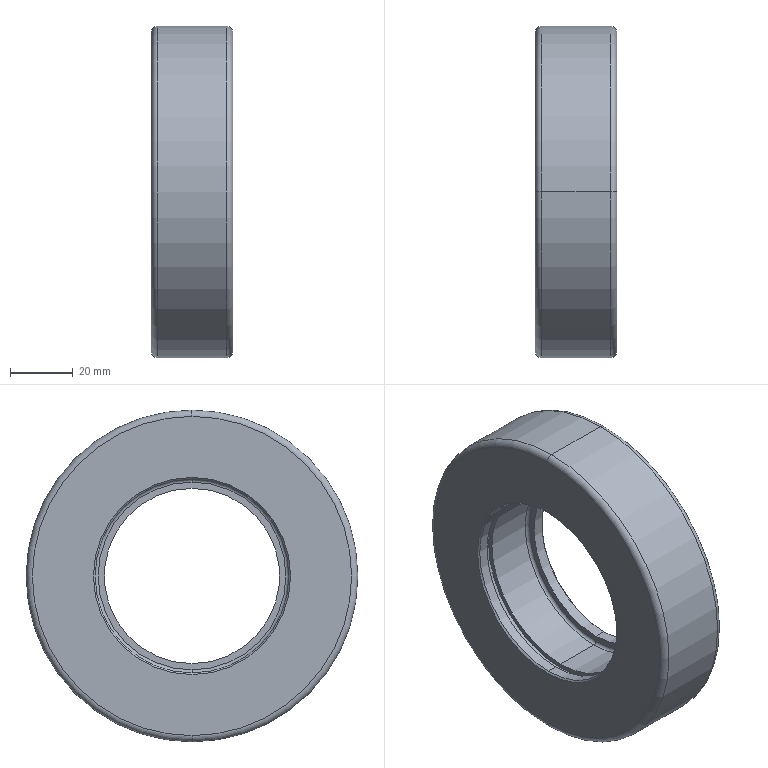Part | STEP file | BT2022003-01-10 Guide wheel A | 1 solid | 25 faces | box 26 x 106 x 106 mm | volume 151941 mm3 | cylinder 10 | torus 6 | plane 5 | cone 4 | commonest cylinder face diameters 62 x4 56 x2 65 x2 106 x2
STEP:
#1=CARTESIAN_POINT('',(0.5,0.,-31.));
#2=VERTEX_POINT('',#1);
#3=CARTESIAN_POINT('',(0.5,0.,31.));
#4=VERTEX_POINT('',#3);
#5=CARTESIAN_POINT('',(0.5,0.,0.));
#6=DIRECTION('',(-1.,0.,0.));
#7=DIRECTION('',(0.,0.,-1.));
#8=AXIS2_PLACEMENT_3D('',#5,#6,#7);
#9=CIRCLE('',#8,31.);
#10=EDGE_CURVE('',#2,#4,#9,.T.);
#11=ORIENTED_EDGE('',*,*,#10,.F.);
#12=CARTESIAN_POINT('',(0.,0.,-31.5));
#13=VERTEX_POINT('',#12);
#14=CARTESIAN_POINT('',(0.5,0.,-31.));
#15=DIRECTION('',(-0.7071,0.,-0.7071));
#16=VECTOR('',#15,1000.);
#17=LINE('',#14,#16);
#18=EDGE_CURVE('',#2,#13,#17,.T.);
#19=ORIENTED_EDGE('',*,*,#18,.T.);
#20=CARTESIAN_POINT('',(0.,0.,31.5));
#21=VERTEX_POINT('',#20);
#22=CARTESIAN_POINT('',(0.,0.,0.));
#23=DIRECTION('',(1.,0.,0.));
#24=DIRECTION('',(0.,0.,-1.));
#25=AXIS2_PLACEMENT_3D('',#22,#23,#24);
#26=CIRCLE('',#25,31.5);
#27=EDGE_CURVE('',#21,#13,#26,.T.);
#28=ORIENTED_EDGE('',*,*,#27,.F.);
#29=CARTESIAN_POINT('',(0.5,0.,31.));
#30=DIRECTION('',(-0.7071,0.,0.7071));
#31=VECTOR('',#30,1000.);
#32=LINE('',#29,#31);
#33=EDGE_CURVE('',#4,#21,#32,.T.);
#34=ORIENTED_EDGE('',*,*,#33,.F.);
#35=EDGE_LOOP('',(#11,#19,#28,#34));
#36=FACE_OUTER_BOUND('',#35,.T.);
#37=CARTESIAN_POINT('',(0.5,0.,0.));
#38=DIRECTION('',(-1.,0.,0.));
#39=DIRECTION('',(0.,0.,1.));
#40=AXIS2_PLACEMENT_3D('',#37,#38,#39);
#41=CONICAL_SURFACE('',#40,31.,0.7854);
#42=ADVANCED_FACE('',(#36),#41,.F.);
#43=CARTESIAN_POINT('',(25.5,0.,28.));
#44=VERTEX_POINT('',#43);
#45=CARTESIAN_POINT('',(25.5,0.,-28.));
#46=VERTEX_POINT('',#45);
#47=CARTESIAN_POINT('',(25.5,0.,0.));
#48=DIRECTION('',(1.,0.,0.));
#49=DIRECTION('',(0.,0.,1.));
#50=AXIS2_PLACEMENT_3D('',#47,#48,#49);
#51=CIRCLE('',#50,28.);
#52=EDGE_CURVE('',#44,#46,#51,.T.);
#53=ORIENTED_EDGE('',*,*,#52,.F.);
#54=CARTESIAN_POINT('',(26.,0.,28.5));
#55=VERTEX_POINT('',#54);
#56=CARTESIAN_POINT('',(26.,0.,28.5));
#57=DIRECTION('',(0.7071,0.,0.7071));
#58=VECTOR('',#57,1000.);
#59=LINE('',#56,#58);
#60=EDGE_CURVE('',#44,#55,#59,.T.);
#61=ORIENTED_EDGE('',*,*,#60,.T.);
#62=CARTESIAN_POINT('',(26.,0.,-28.5));
#63=VERTEX_POINT('',#62);
#64=CARTESIAN_POINT('',(26.,0.,0.));
#65=DIRECTION('',(-1.,0.,0.));
#66=DIRECTION('',(0.,0.,1.));
#67=AXIS2_PLACEMENT_3D('',#64,#65,#66);
#68=CIRCLE('',#67,28.5);
#69=EDGE_CURVE('',#63,#55,#68,.T.);
#70=ORIENTED_EDGE('',*,*,#69,.F.);
#71=CARTESIAN_POINT('',(26.,0.,-28.5));
#72=DIRECTION('',(0.7071,0.,-0.7071));
#73=VECTOR('',#72,1000.);
#74=LINE('',#71,#73);
#75=EDGE_CURVE('',#46,#63,#74,.T.);
#76=ORIENTED_EDGE('',*,*,#75,.F.);
#77=EDGE_LOOP('',(#53,#61,#70,#76));
#78=FACE_OUTER_BOUND('',#77,.T.);
#79=CARTESIAN_POINT('',(26.,0.,0.));
#80=DIRECTION('',(1.,0.,0.));
#81=DIRECTION('',(0.,0.,-1.));
#82=AXIS2_PLACEMENT_3D('',#79,#80,#81);
#83=CONICAL_SURFACE('',#82,28.5,0.7854);
#84=ADVANCED_FACE('',(#78),#83,.F.);
#85=CARTESIAN_POINT('',(26.,0.,-51.));
#86=VERTEX_POINT('',#85);
#87=CARTESIAN_POINT('',(26.,0.,51.));
#88=VERTEX_POINT('',#87);
#89=CARTESIAN_POINT('',(26.,0.,0.));
#90=DIRECTION('',(1.,0.,0.));
#91=DIRECTION('',(0.,0.,1.));
#92=AXIS2_PLACEMENT_3D('',#89,#90,#91);
#93=CIRCLE('',#92,51.);
#94=EDGE_CURVE('',#86,#88,#93,.T.);
#95=ORIENTED_EDGE('',*,*,#94,.F.);
#96=CARTESIAN_POINT('',(24.,0.,-53.));
#97=VERTEX_POINT('',#96);
#98=CARTESIAN_POINT('',(24.,0.,-51.));
#99=DIRECTION('',(0.,1.,0.));
#100=DIRECTION('',(0.,0.,1.));
#101=AXIS2_PLACEMENT_3D('',#98,#99,#100);
#102=CIRCLE('',#101,2.);
#103=EDGE_CURVE('',#86,#97,#102,.T.);
#104=ORIENTED_EDGE('',*,*,#103,.T.);
#105=CARTESIAN_POINT('',(24.,0.,53.));
#106=VERTEX_POINT('',#105);
#107=CARTESIAN_POINT('',(24.,0.,0.));
#108=DIRECTION('',(-1.,0.,0.));
#109=DIRECTION('',(0.,0.,1.));
#110=AXIS2_PLACEMENT_3D('',#107,#108,#109);
#111=CIRCLE('',#110,53.);
#112=EDGE_CURVE('',#106,#97,#111,.T.);
#113=ORIENTED_EDGE('',*,*,#112,.F.);
#114=CARTESIAN_POINT('',(24.,0.,51.));
#115=DIRECTION('',(0.,-1.,0.));
#116=DIRECTION('',(0.,0.,-1.));
#117=AXIS2_PLACEMENT_3D('',#114,#115,#116);
#118=CIRCLE('',#117,2.);
#119=EDGE_CURVE('',#88,#106,#118,.T.);
#120=ORIENTED_EDGE('',*,*,#119,.F.);
#121=EDGE_LOOP('',(#95,#104,#113,#120));
#122=FACE_OUTER_BOUND('',#121,.T.);
#123=CARTESIAN_POINT('',(24.,0.,0.));
#124=DIRECTION('',(-1.,0.,0.));
#125=DIRECTION('',(0.,0.,1.));
#126=AXIS2_PLACEMENT_3D('',#123,#124,#125);
#127=TOROIDAL_SURFACE('',#126,51.,2.);
#128=ADVANCED_FACE('',(#122),#127,.T.);
#129=CARTESIAN_POINT('',(0.,0.,51.));
#130=VERTEX_POINT('',#129);
#131=CARTESIAN_POINT('',(0.,0.,-51.));
#132=VERTEX_POINT('',#131);
#133=CARTESIAN_POINT('',(0.,0.,0.));
#134=DIRECTION('',(-1.,0.,0.));
#135=DIRECTION('',(0.,0.,-1.));
#136=AXIS2_PLACEMENT_3D('',#133,#134,#135);
#137=CIRCLE('',#136,51.);
#138=EDGE_CURVE('',#130,#132,#137,.T.);
#139=ORIENTED_EDGE('',*,*,#138,.F.);
#140=CARTESIAN_POINT('',(2.,0.,53.));
#141=VERTEX_POINT('',#140);
#142=CARTESIAN_POINT('',(2.,0.,51.));
#143=DIRECTION('',(0.,1.,0.));
#144=DIRECTION('',(0.,0.,1.));
#145=AXIS2_PLACEMENT_3D('',#142,#143,#144);
#146=CIRCLE('',#145,2.);
#147=EDGE_CURVE('',#130,#141,#146,.T.);
#148=ORIENTED_EDGE('',*,*,#147,.T.);
#149=CARTESIAN_POINT('',(2.,0.,-53.));
#150=VERTEX_POINT('',#149);
#151=CARTESIAN_POINT('',(2.,0.,0.));
#152=DIRECTION('',(1.,0.,0.));
#153=DIRECTION('',(0.,0.,-1.));
#154=AXIS2_PLACEMENT_3D('',#151,#152,#153);
#155=CIRCLE('',#154,53.);
#156=EDGE_CURVE('',#150,#141,#155,.T.);
#157=ORIENTED_EDGE('',*,*,#156,.F.);
#158=CARTESIAN_POINT('',(2.,0.,-51.));
#159=DIRECTION('',(0.,-1.,0.));
#160=DIRECTION('',(0.,0.,-1.));
#161=AXIS2_PLACEMENT_3D('',#158,#159,#160);
#162=CIRCLE('',#161,2.);
#163=EDGE_CURVE('',#132,#150,#162,.T.);
#164=ORIENTED_EDGE('',*,*,#163,.F.);
#165=EDGE_LOOP('',(#139,#148,#157,#164));
#166=FACE_OUTER_BOUND('',#165,.T.);
#167=CARTESIAN_POINT('',(2.,0.,0.));
#168=DIRECTION('',(1.,0.,0.));
#169=DIRECTION('',(0.,0.,-1.));
#170=AXIS2_PLACEMENT_3D('',#167,#168,#169);
#171=TOROIDAL_SURFACE('',#170,51.,2.);
#172=ADVANCED_FACE('',(#166),#171,.T.);
#173=ORIENTED_EDGE('',*,*,#52,.T.);
#174=CARTESIAN_POINT('',(22.,0.,-28.));
#175=VERTEX_POINT('',#174);
#176=CARTESIAN_POINT('',(0.,0.,-28.));
#177=DIRECTION('',(-1.,0.,0.));
#178=VECTOR('',#177,1000.);
#179=LINE('',#176,#178);
#180=EDGE_CURVE('',#46,#175,#179,.T.);
#181=ORIENTED_EDGE('',*,*,#180,.T.);
#182=CARTESIAN_POINT('',(22.,0.,28.));
#183=VERTEX_POINT('',#182);
#184=CARTESIAN_POINT('',(22.,0.,0.));
#185=DIRECTION('',(-1.,0.,0.));
#186=DIRECTION('',(0.,0.,1.));
#187=AXIS2_PLACEMENT_3D('',#184,#185,#186);
#188=CIRCLE('',#187,28.);
#189=EDGE_CURVE('',#175,#183,#188,.T.);
#190=ORIENTED_EDGE('',*,*,#189,.T.);
#191=CARTESIAN_POINT('',(0.,0.,28.));
#192=DIRECTION('',(-1.,0.,0.));
#193=VECTOR('',#192,1000.);
#194=LINE('',#191,#193);
#195=EDGE_CURVE('',#44,#183,#194,.T.);
#196=ORIENTED_EDGE('',*,*,#195,.F.);
#197=EDGE_LOOP('',(#173,#181,#190,#196));
#198=FACE_OUTER_BOUND('',#197,.T.);
#199=CARTESIAN_POINT('',(0.,0.,0.));
#200=DIRECTION('',(-1.,0.,0.));
#201=DIRECTION('',(0.,0.,1.));
#202=AXIS2_PLACEMENT_3D('',#199,#200,#201);
#203=CYLINDRICAL_SURFACE('',#202,28.);
#204=ADVANCED_FACE('',(#198),#203,.F.);
#205=ORIENTED_EDGE('',*,*,#112,.T.);
#206=CARTESIAN_POINT('',(0.,0.,-53.));
#207=DIRECTION('',(-1.,0.,0.));
#208=VECTOR('',#207,1000.);
#209=LINE('',#206,#208);
#210=EDGE_CURVE('',#97,#150,#209,.T.);
#211=ORIENTED_EDGE('',*,*,#210,.T.);
#212=ORIENTED_EDGE('',*,*,#156,.T.);
#213=CARTESIAN_POINT('',(0.,0.,53.));
#214=DIRECTION('',(-1.,0.,0.));
#215=VECTOR('',#214,1000.);
#216=LINE('',#213,#215);
#217=EDGE_CURVE('',#106,#141,#216,.T.);
#218=ORIENTED_EDGE('',*,*,#217,.F.);
#219=EDGE_LOOP('',(#205,#211,#212,#218));
#220=FACE_OUTER_BOUND('',#219,.T.);
#221=CARTESIAN_POINT('',(0.,0.,0.));
#222=DIRECTION('',(-1.,0.,0.));
#223=DIRECTION('',(0.,0.,1.));
#224=AXIS2_PLACEMENT_3D('',#221,#222,#223);
#225=CYLINDRICAL_SURFACE('',#224,53.);
#226=ADVANCED_FACE('',(#220),#225,.T.);
#227=CARTESIAN_POINT('',(3.8,0.,-31.));
#228=VERTEX_POINT('',#227);
#229=CARTESIAN_POINT('',(3.8,0.,31.));
#230=VERTEX_POINT('',#229);
#231=CARTESIAN_POINT('',(3.8,0.,0.));
#232=DIRECTION('',(-1.,0.,0.));
#233=DIRECTION('',(0.,0.,1.));
#234=AXIS2_PLACEMENT_3D('',#231,#232,#233);
#235=CIRCLE('',#234,31.);
#236=EDGE_CURVE('',#228,#230,#235,.T.);
#237=ORIENTED_EDGE('',*,*,#236,.F.);
#238=CARTESIAN_POINT('',(0.,0.,-31.));
#239=DIRECTION('',(-1.,0.,0.));
#240=VECTOR('',#239,1000.);
#241=LINE('',#238,#240);
#242=EDGE_CURVE('',#228,#2,#241,.T.);
#243=ORIENTED_EDGE('',*,*,#242,.T.);
#244=ORIENTED_EDGE('',*,*,#10,.T.);
#245=CARTESIAN_POINT('',(0.,0.,31.));
#246=DIRECTION('',(-1.,0.,0.));
#247=VECTOR('',#246,1000.);
#248=LINE('',#245,#247);
#249=EDGE_CURVE('',#230,#4,#248,.T.);
#250=ORIENTED_EDGE('',*,*,#249,.F.);
#251=EDGE_LOOP('',(#237,#243,#244,#250));
#252=FACE_OUTER_BOUND('',#251,.T.);
#253=CARTESIAN_POINT('',(0.,0.,0.));
#254=DIRECTION('',(-1.,0.,0.));
#255=DIRECTION('',(0.,0.,1.));
#256=AXIS2_PLACEMENT_3D('',#253,#254,#255);
#257=CYLINDRICAL_SURFACE('',#256,31.);
#258=ADVANCED_FACE('',(#252),#257,.F.);
#259=CARTESIAN_POINT('',(6.,0.,-32.5));
#260=VERTEX_POINT('',#259);
#261=CARTESIAN_POINT('',(6.,0.,32.5));
#262=VERTEX_POINT('',#261);
#263=CARTESIAN_POINT('',(6.,0.,0.));
#264=DIRECTION('',(-1.,0.,0.));
#265=DIRECTION('',(0.,0.,1.));
#266=AXIS2_PLACEMENT_3D('',#263,#264,#265);
#267=CIRCLE('',#266,32.5);
#268=EDGE_CURVE('',#260,#262,#267,.T.);
#269=ORIENTED_EDGE('',*,*,#268,.F.);
#270=CARTESIAN_POINT('',(3.8,0.,-32.5));
#271=VERTEX_POINT('',#270);
#272=CARTESIAN_POINT('',(0.,0.,-32.5));
#273=DIRECTION('',(-1.,0.,0.));
#274=VECTOR('',#273,1000.);
#275=LINE('',#272,#274);
#276=EDGE_CURVE('',#260,#271,#275,.T.);
#277=ORIENTED_EDGE('',*,*,#276,.T.);
#278=CARTESIAN_POINT('',(3.8,0.,32.5));
#279=VERTEX_POINT('',#278);
#280=CARTESIAN_POINT('',(3.8,0.,0.));
#281=DIRECTION('',(-1.,0.,0.));
#282=DIRECTION('',(0.,0.,1.));
#283=AXIS2_PLACEMENT_3D('',#280,#281,#282);
#284=CIRCLE('',#283,32.5);
#285=EDGE_CURVE('',#271,#279,#284,.T.);
#286=ORIENTED_EDGE('',*,*,#285,.T.);
#287=CARTESIAN_POINT('',(0.,0.,32.5));
#288=DIRECTION('',(-1.,0.,0.));
#289=VECTOR('',#288,1000.);
#290=LINE('',#287,#289);
#291=EDGE_CURVE('',#262,#279,#290,.T.);
#292=ORIENTED_EDGE('',*,*,#291,.F.);
#293=EDGE_LOOP('',(#269,#277,#286,#292));
#294=FACE_OUTER_BOUND('',#293,.T.);
#295=CARTESIAN_POINT('',(0.,0.,0.));
#296=DIRECTION('',(-1.,0.,0.));
#297=DIRECTION('',(0.,0.,1.));
#298=AXIS2_PLACEMENT_3D('',#295,#296,#297);
#299=CYLINDRICAL_SURFACE('',#298,32.5);
#300=ADVANCED_FACE('',(#294),#299,.F.);
#301=CARTESIAN_POINT('',(21.,0.,-31.));
#302=VERTEX_POINT('',#301);
#303=CARTESIAN_POINT('',(21.,0.,31.));
#304=VERTEX_POINT('',#303);
#305=CARTESIAN_POINT('',(21.,0.,0.));
#306=DIRECTION('',(-1.,0.,0.));
#307=DIRECTION('',(0.,0.,1.));
#308=AXIS2_PLACEMENT_3D('',#305,#306,#307);
#309=CIRCLE('',#308,31.);
#310=EDGE_CURVE('',#302,#304,#309,.T.);
#311=ORIENTED_EDGE('',*,*,#310,.F.);
#312=CARTESIAN_POINT('',(6.,0.,-31.));
#313=VERTEX_POINT('',#312);
#314=CARTESIAN_POINT('',(0.,0.,-31.));
#315=DIRECTION('',(-1.,0.,0.));
#316=VECTOR('',#315,1000.);
#317=LINE('',#314,#316);
#318=EDGE_CURVE('',#302,#313,#317,.T.);
#319=ORIENTED_EDGE('',*,*,#318,.T.);
#320=CARTESIAN_POINT('',(6.,0.,31.));
#321=VERTEX_POINT('',#320);
#322=CARTESIAN_POINT('',(6.,0.,0.));
#323=DIRECTION('',(-1.,0.,0.));
#324=DIRECTION('',(0.,0.,1.));
#325=AXIS2_PLACEMENT_3D('',#322,#323,#324);
#326=CIRCLE('',#325,31.);
#327=EDGE_CURVE('',#313,#321,#326,.T.);
#328=ORIENTED_EDGE('',*,*,#327,.T.);
#329=CARTESIAN_POINT('',(0.,0.,31.));
#330=DIRECTION('',(-1.,0.,0.));
#331=VECTOR('',#330,1000.);
#332=LINE('',#329,#331);
#333=EDGE_CURVE('',#304,#321,#332,.T.);
#334=ORIENTED_EDGE('',*,*,#333,.F.);
#335=EDGE_LOOP('',(#311,#319,#328,#334));
#336=FACE_OUTER_BOUND('',#335,.T.);
#337=CARTESIAN_POINT('',(0.,0.,0.));
#338=DIRECTION('',(-1.,0.,0.));
#339=DIRECTION('',(0.,0.,1.));
#340=AXIS2_PLACEMENT_3D('',#337,#338,#339);
#341=CYLINDRICAL_SURFACE('',#340,31.);
#342=ADVANCED_FACE('',(#336),#341,.F.);
#343=CARTESIAN_POINT('',(22.,0.,-30.));
#344=VERTEX_POINT('',#343);
#345=CARTESIAN_POINT('',(22.,0.,30.));
#346=VERTEX_POINT('',#345);
#347=CARTESIAN_POINT('',(22.,0.,0.));
#348=DIRECTION('',(-1.,0.,0.));
#349=DIRECTION('',(0.,0.,1.));
#350=AXIS2_PLACEMENT_3D('',#347,#348,#349);
#351=CIRCLE('',#350,30.);
#352=EDGE_CURVE('',#344,#346,#351,.T.);
#353=ORIENTED_EDGE('',*,*,#352,.F.);
#354=CARTESIAN_POINT('',(21.,0.,-30.));
#355=DIRECTION('',(0.,1.,0.));
#356=DIRECTION('',(0.,0.,1.));
#357=AXIS2_PLACEMENT_3D('',#354,#355,#356);
#358=CIRCLE('',#357,1.);
#359=EDGE_CURVE('',#344,#302,#358,.T.);
#360=ORIENTED_EDGE('',*,*,#359,.T.);
#361=ORIENTED_EDGE('',*,*,#310,.T.);
#362=CARTESIAN_POINT('',(21.,0.,30.));
#363=DIRECTION('',(0.,-1.,0.));
#364=DIRECTION('',(0.,0.,-1.));
#365=AXIS2_PLACEMENT_3D('',#362,#363,#364);
#366=CIRCLE('',#365,1.);
#367=EDGE_CURVE('',#346,#304,#366,.T.);
#368=ORIENTED_EDGE('',*,*,#367,.F.);
#369=EDGE_LOOP('',(#353,#360,#361,#368));
#370=FACE_OUTER_BOUND('',#369,.T.);
#371=CARTESIAN_POINT('',(21.,0.,0.));
#372=DIRECTION('',(-1.,0.,0.));
#373=DIRECTION('',(0.,0.,1.));
#374=AXIS2_PLACEMENT_3D('',#371,#372,#373);
#375=TOROIDAL_SURFACE('',#374,30.,1.);
#376=ADVANCED_FACE('',(#370),#375,.F.);
#377=ORIENTED_EDGE('',*,*,#359,.F.);
#378=CARTESIAN_POINT('',(22.,0.,0.));
#379=DIRECTION('',(-1.,0.,0.));
#380=DIRECTION('',(0.,0.,1.));
#381=AXIS2_PLACEMENT_3D('',#378,#379,#380);
#382=CIRCLE('',#381,30.);
#383=EDGE_CURVE('',#346,#344,#382,.T.);
#384=ORIENTED_EDGE('',*,*,#383,.F.);
#385=ORIENTED_EDGE('',*,*,#367,.T.);
#386=CARTESIAN_POINT('',(21.,0.,0.));
#387=DIRECTION('',(-1.,0.,0.));
#388=DIRECTION('',(0.,0.,1.));
#389=AXIS2_PLACEMENT_3D('',#386,#387,#388);
#390=CIRCLE('',#389,31.);
#391=EDGE_CURVE('',#304,#302,#390,.T.);
#392=ORIENTED_EDGE('',*,*,#391,.T.);
#393=EDGE_LOOP('',(#377,#384,#385,#392));
#394=FACE_OUTER_BOUND('',#393,.T.);
#395=CARTESIAN_POINT('',(21.,0.,0.));
#396=DIRECTION('',(-1.,0.,0.));
#397=DIRECTION('',(0.,0.,1.));
#398=AXIS2_PLACEMENT_3D('',#395,#396,#397);
#399=TOROIDAL_SURFACE('',#398,30.,1.);
#400=ADVANCED_FACE('',(#394),#399,.F.);
#401=ORIENTED_EDGE('',*,*,#318,.F.);
#402=ORIENTED_EDGE('',*,*,#391,.F.);
#403=ORIENTED_EDGE('',*,*,#333,.T.);
#404=CARTESIAN_POINT('',(6.,0.,0.));
#405=DIRECTION('',(-1.,0.,0.));
#406=DIRECTION('',(0.,0.,1.));
#407=AXIS2_PLACEMENT_3D('',#404,#405,#406);
#408=CIRCLE('',#407,31.);
#409=EDGE_CURVE('',#321,#313,#408,.T.);
#410=ORIENTED_EDGE('',*,*,#409,.T.);
#411=EDGE_LOOP('',(#401,#402,#403,#410));
#412=FACE_OUTER_BOUND('',#411,.T.);
#413=CARTESIAN_POINT('',(0.,0.,0.));
#414=DIRECTION('',(-1.,0.,0.));
#415=DIRECTION('',(0.,0.,1.));
#416=AXIS2_PLACEMENT_3D('',#413,#414,#415);
#417=CYLINDRICAL_SURFACE('',#416,31.);
#418=ADVANCED_FACE('',(#412),#417,.F.);
#419=ORIENTED_EDGE('',*,*,#409,.F.);
#420=ORIENTED_EDGE('',*,*,#327,.F.);
#421=EDGE_LOOP('',(#419,#420));
#422=FACE_BOUND('',#421,.T.);
#423=CARTESIAN_POINT('',(6.,0.,0.));
#424=DIRECTION('',(-1.,0.,0.));
#425=DIRECTION('',(0.,0.,1.));
#426=AXIS2_PLACEMENT_3D('',#423,#424,#425);
#427=CIRCLE('',#426,32.5);
#428=EDGE_CURVE('',#262,#260,#427,.T.);
#429=ORIENTED_EDGE('',*,*,#428,.T.);
#430=ORIENTED_EDGE('',*,*,#268,.T.);
#431=EDGE_LOOP('',(#429,#430));
#432=FACE_OUTER_BOUND('',#431,.T.);
#433=CARTESIAN_POINT('',(6.,32.5,0.));
#434=DIRECTION('',(1.,0.,0.));
#435=DIRECTION('',(0.,0.,-1.));
#436=AXIS2_PLACEMENT_3D('',#433,#434,#435);
#437=PLANE('',#436);
#438=ADVANCED_FACE('',(#422,#432),#437,.F.);
#439=ORIENTED_EDGE('',*,*,#276,.F.);
#440=ORIENTED_EDGE('',*,*,#428,.F.);
#441=ORIENTED_EDGE('',*,*,#291,.T.);
#442=CARTESIAN_POINT('',(3.8,0.,0.));
#443=DIRECTION('',(-1.,0.,0.));
#444=DIRECTION('',(0.,0.,1.));
#445=AXIS2_PLACEMENT_3D('',#442,#443,#444);
#446=CIRCLE('',#445,32.5);
#447=EDGE_CURVE('',#279,#271,#446,.T.);
#448=ORIENTED_EDGE('',*,*,#447,.T.);
#449=EDGE_LOOP('',(#439,#440,#441,#448));
#450=FACE_OUTER_BOUND('',#449,.T.);
#451=CARTESIAN_POINT('',(0.,0.,0.));
#452=DIRECTION('',(-1.,0.,0.));
#453=DIRECTION('',(0.,0.,1.));
#454=AXIS2_PLACEMENT_3D('',#451,#452,#453);
#455=CYLINDRICAL_SURFACE('',#454,32.5);
#456=ADVANCED_FACE('',(#450),#455,.F.);
#457=ORIENTED_EDGE('',*,*,#447,.F.);
#458=ORIENTED_EDGE('',*,*,#285,.F.);
#459=EDGE_LOOP('',(#457,#458));
#460=FACE_OUTER_BOUND('',#459,.T.);
#461=CARTESIAN_POINT('',(3.8,0.,0.));
#462=DIRECTION('',(-1.,0.,0.));
#463=DIRECTION('',(0.,0.,1.));
#464=AXIS2_PLACEMENT_3D('',#461,#462,#463);
#465=CIRCLE('',#464,31.);
#466=EDGE_CURVE('',#230,#228,#465,.T.);
#467=ORIENTED_EDGE('',*,*,#466,.T.);
#468=ORIENTED_EDGE('',*,*,#236,.T.);
#469=EDGE_LOOP('',(#467,#468));
#470=FACE_BOUND('',#469,.T.);
#471=CARTESIAN_POINT('',(3.8,31.,0.));
#472=DIRECTION('',(-1.,0.,0.));
#473=DIRECTION('',(0.,0.,1.));
#474=AXIS2_PLACEMENT_3D('',#471,#472,#473);
#475=PLANE('',#474);
#476=ADVANCED_FACE('',(#460,#470),#475,.F.);
#477=ORIENTED_EDGE('',*,*,#242,.F.);
#478=ORIENTED_EDGE('',*,*,#466,.F.);
#479=ORIENTED_EDGE('',*,*,#249,.T.);
#480=CARTESIAN_POINT('',(0.5,0.,0.));
#481=DIRECTION('',(-1.,0.,0.));
#482=DIRECTION('',(0.,0.,-1.));
#483=AXIS2_PLACEMENT_3D('',#480,#481,#482);
#484=CIRCLE('',#483,31.);
#485=EDGE_CURVE('',#4,#2,#484,.T.);
#486=ORIENTED_EDGE('',*,*,#485,.T.);
#487=EDGE_LOOP('',(#477,#478,#479,#486));
#488=FACE_OUTER_BOUND('',#487,.T.);
#489=CARTESIAN_POINT('',(0.,0.,0.));
#490=DIRECTION('',(-1.,0.,0.));
#491=DIRECTION('',(0.,0.,1.));
#492=AXIS2_PLACEMENT_3D('',#489,#490,#491);
#493=CYLINDRICAL_SURFACE('',#492,31.);
#494=ADVANCED_FACE('',(#488),#493,.F.);
#495=ORIENTED_EDGE('',*,*,#27,.T.);
#496=CARTESIAN_POINT('',(0.,0.,0.));
#497=DIRECTION('',(1.,0.,0.));
#498=DIRECTION('',(0.,0.,-1.));
#499=AXIS2_PLACEMENT_3D('',#496,#497,#498);
#500=CIRCLE('',#499,31.5);
#501=EDGE_CURVE('',#13,#21,#500,.T.);
#502=ORIENTED_EDGE('',*,*,#501,.T.);
#503=EDGE_LOOP('',(#495,#502));
#504=FACE_BOUND('',#503,.T.);
#505=CARTESIAN_POINT('',(0.,0.,0.));
#506=DIRECTION('',(-1.,0.,0.));
#507=DIRECTION('',(0.,0.,-1.));
#508=AXIS2_PLACEMENT_3D('',#505,#506,#507);
#509=CIRCLE('',#508,51.);
#510=EDGE_CURVE('',#132,#130,#509,.T.);
#511=ORIENTED_EDGE('',*,*,#510,.T.);
#512=ORIENTED_EDGE('',*,*,#138,.T.);
#513=EDGE_LOOP('',(#511,#512));
#514=FACE_OUTER_BOUND('',#513,.T.);
#515=CARTESIAN_POINT('',(0.,53.,0.));
#516=DIRECTION('',(1.,0.,0.));
#517=DIRECTION('',(0.,0.,-1.));
#518=AXIS2_PLACEMENT_3D('',#515,#516,#517);
#519=PLANE('',#518);
#520=ADVANCED_FACE('',(#504,#514),#519,.F.);
#521=ORIENTED_EDGE('',*,*,#210,.F.);
#522=CARTESIAN_POINT('',(24.,0.,0.));
#523=DIRECTION('',(-1.,0.,0.));
#524=DIRECTION('',(0.,0.,1.));
#525=AXIS2_PLACEMENT_3D('',#522,#523,#524);
#526=CIRCLE('',#525,53.);
#527=EDGE_CURVE('',#97,#106,#526,.T.);
#528=ORIENTED_EDGE('',*,*,#527,.T.);
#529=ORIENTED_EDGE('',*,*,#217,.T.);
#530=CARTESIAN_POINT('',(2.,0.,0.));
#531=DIRECTION('',(1.,0.,0.));
#532=DIRECTION('',(0.,0.,-1.));
#533=AXIS2_PLACEMENT_3D('',#530,#531,#532);
#534=CIRCLE('',#533,53.);
#535=EDGE_CURVE('',#141,#150,#534,.T.);
#536=ORIENTED_EDGE('',*,*,#535,.T.);
#537=EDGE_LOOP('',(#521,#528,#529,#536));
#538=FACE_OUTER_BOUND('',#537,.T.);
#539=CARTESIAN_POINT('',(0.,0.,0.));
#540=DIRECTION('',(-1.,0.,0.));
#541=DIRECTION('',(0.,0.,1.));
#542=AXIS2_PLACEMENT_3D('',#539,#540,#541);
#543=CYLINDRICAL_SURFACE('',#542,53.);
#544=ADVANCED_FACE('',(#538),#543,.T.);
#545=ORIENTED_EDGE('',*,*,#69,.T.);
#546=CARTESIAN_POINT('',(26.,0.,0.));
#547=DIRECTION('',(-1.,0.,0.));
#548=DIRECTION('',(0.,0.,1.));
#549=AXIS2_PLACEMENT_3D('',#546,#547,#548);
#550=CIRCLE('',#549,28.5);
#551=EDGE_CURVE('',#55,#63,#550,.T.);
#552=ORIENTED_EDGE('',*,*,#551,.T.);
#553=EDGE_LOOP('',(#545,#552));
#554=FACE_BOUND('',#553,.T.);
#555=CARTESIAN_POINT('',(26.,0.,0.));
#556=DIRECTION('',(1.,0.,0.));
#557=DIRECTION('',(0.,0.,1.));
#558=AXIS2_PLACEMENT_3D('',#555,#556,#557);
#559=CIRCLE('',#558,51.);
#560=EDGE_CURVE('',#88,#86,#559,.T.);
#561=ORIENTED_EDGE('',*,*,#560,.T.);
#562=ORIENTED_EDGE('',*,*,#94,.T.);
#563=EDGE_LOOP('',(#561,#562));
#564=FACE_OUTER_BOUND('',#563,.T.);
#565=CARTESIAN_POINT('',(26.,28.,0.));
#566=DIRECTION('',(-1.,0.,0.));
#567=DIRECTION('',(0.,0.,1.));
#568=AXIS2_PLACEMENT_3D('',#565,#566,#567);
#569=PLANE('',#568);
#570=ADVANCED_FACE('',(#554,#564),#569,.F.);
#571=ORIENTED_EDGE('',*,*,#180,.F.);
#572=CARTESIAN_POINT('',(25.5,0.,0.));
#573=DIRECTION('',(1.,0.,0.));
#574=DIRECTION('',(0.,0.,1.));
#575=AXIS2_PLACEMENT_3D('',#572,#573,#574);
#576=CIRCLE('',#575,28.);
#577=EDGE_CURVE('',#46,#44,#576,.T.);
#578=ORIENTED_EDGE('',*,*,#577,.T.);
#579=ORIENTED_EDGE('',*,*,#195,.T.);
#580=CARTESIAN_POINT('',(22.,0.,0.));
#581=DIRECTION('',(-1.,0.,0.));
#582=DIRECTION('',(0.,0.,1.));
#583=AXIS2_PLACEMENT_3D('',#580,#581,#582);
#584=CIRCLE('',#583,28.);
#585=EDGE_CURVE('',#183,#175,#584,.T.);
#586=ORIENTED_EDGE('',*,*,#585,.T.);
#587=EDGE_LOOP('',(#571,#578,#579,#586));
#588=FACE_OUTER_BOUND('',#587,.T.);
#589=CARTESIAN_POINT('',(0.,0.,0.));
#590=DIRECTION('',(-1.,0.,0.));
#591=DIRECTION('',(0.,0.,1.));
#592=AXIS2_PLACEMENT_3D('',#589,#590,#591);
#593=CYLINDRICAL_SURFACE('',#592,28.);
#594=ADVANCED_FACE('',(#588),#593,.F.);
#595=ORIENTED_EDGE('',*,*,#585,.F.);
#596=ORIENTED_EDGE('',*,*,#189,.F.);
#597=EDGE_LOOP('',(#595,#596));
#598=FACE_BOUND('',#597,.T.);
#599=ORIENTED_EDGE('',*,*,#383,.T.);
#600=ORIENTED_EDGE('',*,*,#352,.T.);
#601=EDGE_LOOP('',(#599,#600));
#602=FACE_OUTER_BOUND('',#601,.T.);
#603=CARTESIAN_POINT('',(22.,30.,0.));
#604=DIRECTION('',(1.,0.,0.));
#605=DIRECTION('',(0.,0.,-1.));
#606=AXIS2_PLACEMENT_3D('',#603,#604,#605);
#607=PLANE('',#606);
#608=ADVANCED_FACE('',(#598,#602),#607,.F.);
#609=ORIENTED_EDGE('',*,*,#147,.F.);
#610=ORIENTED_EDGE('',*,*,#510,.F.);
#611=ORIENTED_EDGE('',*,*,#163,.T.);
#612=ORIENTED_EDGE('',*,*,#535,.F.);
#613=EDGE_LOOP('',(#609,#610,#611,#612));
#614=FACE_OUTER_BOUND('',#613,.T.);
#615=CARTESIAN_POINT('',(2.,0.,0.));
#616=DIRECTION('',(1.,0.,0.));
#617=DIRECTION('',(0.,0.,-1.));
#618=AXIS2_PLACEMENT_3D('',#615,#616,#617);
#619=TOROIDAL_SURFACE('',#618,51.,2.);
#620=ADVANCED_FACE('',(#614),#619,.T.);
#621=ORIENTED_EDGE('',*,*,#103,.F.);
#622=ORIENTED_EDGE('',*,*,#560,.F.);
#623=ORIENTED_EDGE('',*,*,#119,.T.);
#624=ORIENTED_EDGE('',*,*,#527,.F.);
#625=EDGE_LOOP('',(#621,#622,#623,#624));
#626=FACE_OUTER_BOUND('',#625,.T.);
#627=CARTESIAN_POINT('',(24.,0.,0.));
#628=DIRECTION('',(-1.,0.,0.));
#629=DIRECTION('',(0.,0.,1.));
#630=AXIS2_PLACEMENT_3D('',#627,#628,#629);
#631=TOROIDAL_SURFACE('',#630,51.,2.);
#632=ADVANCED_FACE('',(#626),#631,.T.);
#633=ORIENTED_EDGE('',*,*,#60,.F.);
#634=ORIENTED_EDGE('',*,*,#577,.F.);
#635=ORIENTED_EDGE('',*,*,#75,.T.);
#636=ORIENTED_EDGE('',*,*,#551,.F.);
#637=EDGE_LOOP('',(#633,#634,#635,#636));
#638=FACE_OUTER_BOUND('',#637,.T.);
#639=CARTESIAN_POINT('',(26.,0.,0.));
#640=DIRECTION('',(1.,0.,0.));
#641=DIRECTION('',(0.,0.,-1.));
#642=AXIS2_PLACEMENT_3D('',#639,#640,#641);
#643=CONICAL_SURFACE('',#642,28.5,0.7854);
#644=ADVANCED_FACE('',(#638),#643,.F.);
#645=ORIENTED_EDGE('',*,*,#18,.F.);
#646=ORIENTED_EDGE('',*,*,#485,.F.);
#647=ORIENTED_EDGE('',*,*,#33,.T.);
#648=ORIENTED_EDGE('',*,*,#501,.F.);
#649=EDGE_LOOP('',(#645,#646,#647,#648));
#650=FACE_OUTER_BOUND('',#649,.T.);
#651=CARTESIAN_POINT('',(0.5,0.,0.));
#652=DIRECTION('',(-1.,0.,0.));
#653=DIRECTION('',(0.,0.,1.));
#654=AXIS2_PLACEMENT_3D('',#651,#652,#653);
#655=CONICAL_SURFACE('',#654,31.,0.7854);
#656=ADVANCED_FACE('',(#650),#655,.F.);
#657=CLOSED_SHELL('',(#42,#84,#128,#172,#204,#226,#258,#300,#342,#376,#400,#418,#438,#456,#476,#494,#520,#544,#570,#594,#608,#620,#632,#644,#656));
#658=MANIFOLD_SOLID_BREP('',#657);
#659=CARTESIAN_POINT('',(0.,0.,0.));
#660=DIRECTION('',(0.,0.,1.));
#661=DIRECTION('',(1.,0.,0.));
#662=AXIS2_PLACEMENT_3D('',#659,#660,#661);
#663=(LENGTH_UNIT()NAMED_UNIT(*)SI_UNIT(.MILLI.,.METRE.));
#664=UNCERTAINTY_MEASURE_WITH_UNIT(LENGTH_MEASURE(0.00001),#663,'','');
#665=(NAMED_UNIT(*)PLANE_ANGLE_UNIT()SI_UNIT($,.RADIAN.));
#666=(NAMED_UNIT(*)SI_UNIT($,.STERADIAN.)SOLID_ANGLE_UNIT());
#667=(GEOMETRIC_REPRESENTATION_CONTEXT(3)GLOBAL_UNCERTAINTY_ASSIGNED_CONTEXT((#664))GLOBAL_UNIT_ASSIGNED_CONTEXT((#663,#665,#666))REPRESENTATION_CONTEXT('',''));
#668=ADVANCED_BREP_SHAPE_REPRESENTATION('',(#658,#662),#667);